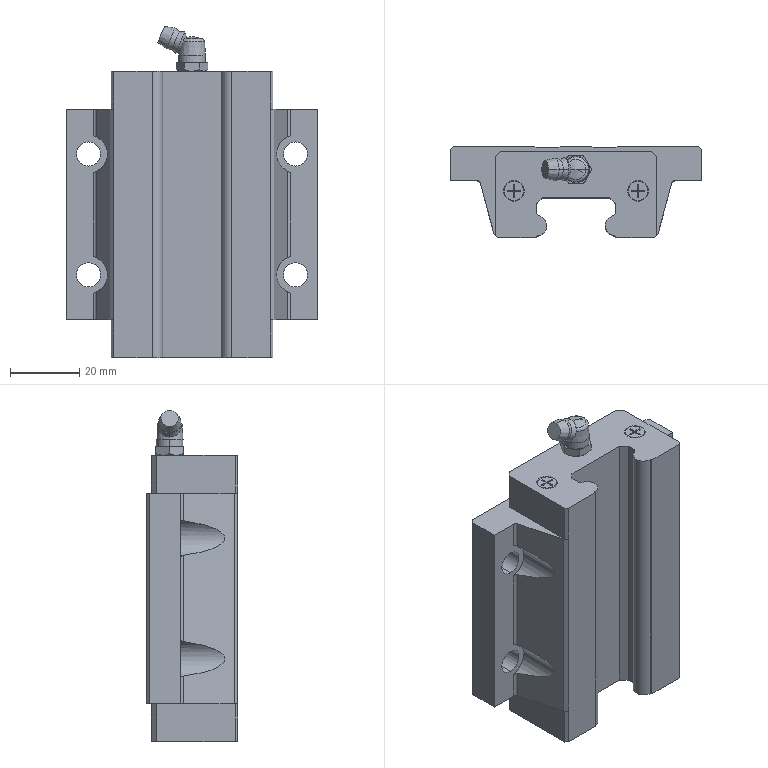Part | STEP file | 0244_Z_004_SX2W33-1240_2 | 1 solid | 188 faces | box 73 x 26.5 x 96 mm | volume 100678 mm3 | plane 99 | cylinder 61 | cone 26 | spline 2 | commonest cylinder face diameters 3.92 x20 6 x11 5.6 x8 7 x8 2 x6 11 x4